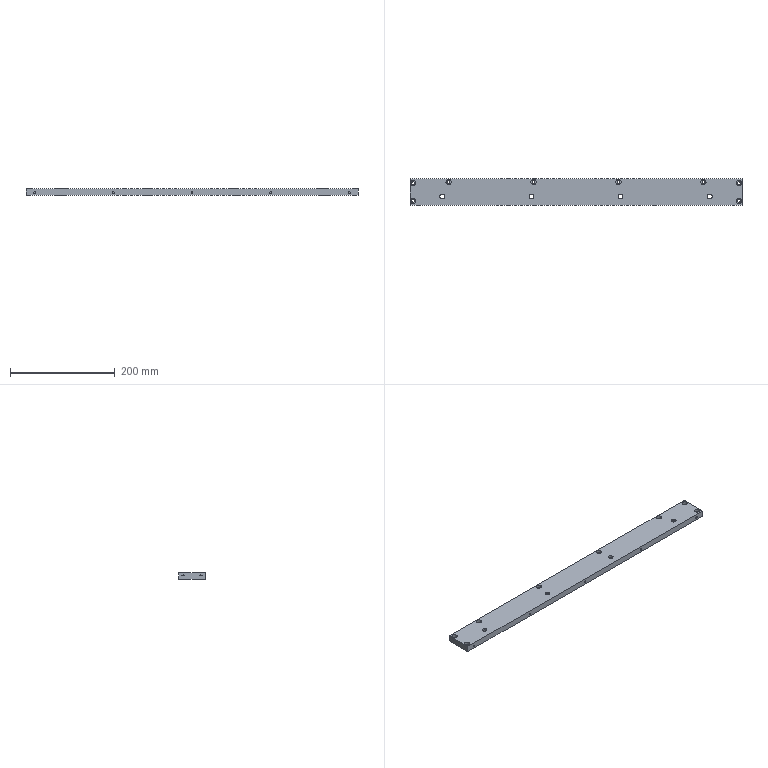Part | STEP file | Shim lower mounting plate 2 | 1 solid | 81 faces | box 633 x 50 x 12 mm | volume 367777 mm3 | cylinder 58 | plane 23 | commonest cylinder face diameters 5.5 x16 10 x16 3.3 x10 9 x8 15 x8